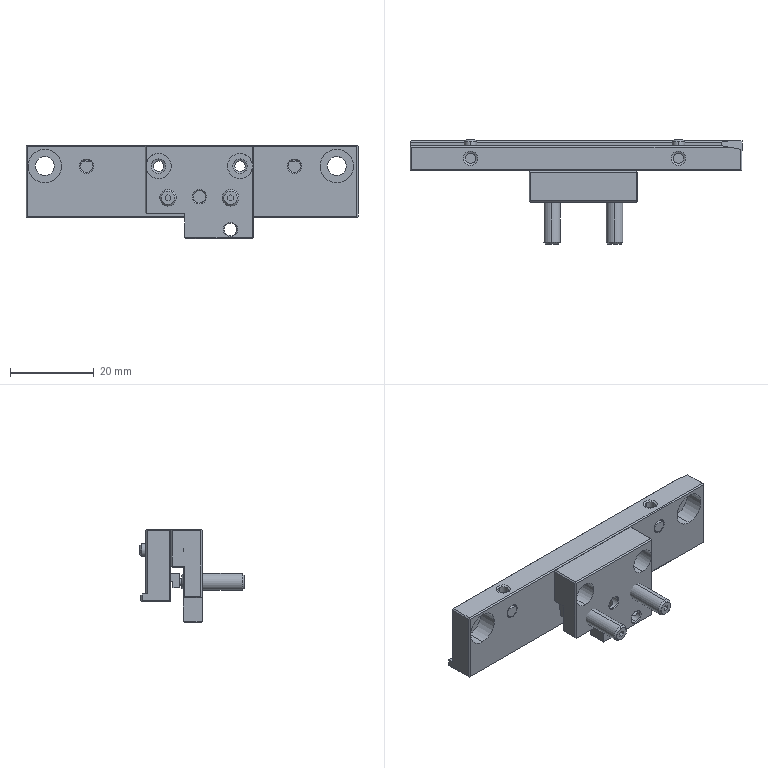Part | NX | 8 solids | 205 faces | box 79.5 x 25.105 x 22.4 mm | volume 11082 mm3 | plane 104 | cylinder 62 | cone 36 | sphere 3 | commonest cylinder face diameters 2.5 x12 3 x12 1.6 x6 3.2 x6 4 x6 3.3 x4